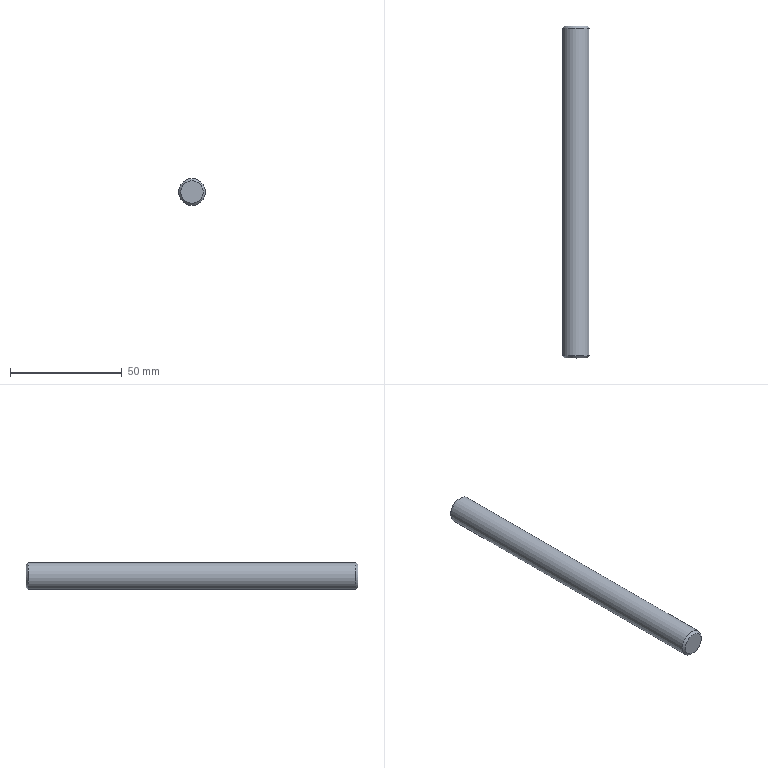Part | NX | features solid 2 | 1 solid | 5 faces | box 12 x 148.5 x 12 mm | volume 16759 mm3 | plane 2 | cone 2 | cylinder 1 | commonest cylinder face diameters 12 x1
STEP:
#1=CARTESIAN_POINT('',(0.,611.5,-123.));
#2=VERTEX_POINT('',#1);
#3=CARTESIAN_POINT('',(0.,611.5,-117.));
#4=DIRECTION('',(0.,-1.,0.));
#5=DIRECTION('',(0.,0.,-1.));
#6=AXIS2_PLACEMENT_3D('',#3,#4,#5);
#7=CIRCLE('',#6,6.);
#8=EDGE_CURVE('',#2,#2,#7,.F.);
#9=ORIENTED_EDGE('',*,*,#8,.T.);
#10=EDGE_LOOP('',(#9));
#11=FACE_BOUND('',#10,.T.);
#12=CARTESIAN_POINT('',(0.,758.,-123.));
#13=VERTEX_POINT('',#12);
#14=CARTESIAN_POINT('',(0.,758.,-117.));
#15=DIRECTION('',(0.,-1.,0.));
#16=DIRECTION('',(0.,0.,-1.));
#17=AXIS2_PLACEMENT_3D('',#14,#15,#16);
#18=CIRCLE('',#17,6.);
#19=EDGE_CURVE('',#13,#13,#18,.T.);
#20=ORIENTED_EDGE('',*,*,#19,.T.);
#21=EDGE_LOOP('',(#20));
#22=FACE_BOUND('',#21,.T.);
#23=CARTESIAN_POINT('',(0.,611.,-117.));
#24=DIRECTION('',(0.,1.,0.));
#25=DIRECTION('',(0.,0.,1.));
#26=AXIS2_PLACEMENT_3D('',#23,#24,#25);
#27=CYLINDRICAL_SURFACE('',#26,6.);
#28=ADVANCED_FACE('',(#11,#22),#27,.T.);
#29=CARTESIAN_POINT('',(0.,610.5,-122.));
#30=VERTEX_POINT('',#29);
#31=CARTESIAN_POINT('',(0.,610.5,-117.));
#32=DIRECTION('',(0.,-1.,0.));
#33=DIRECTION('',(0.,0.,-1.));
#34=AXIS2_PLACEMENT_3D('',#31,#32,#33);
#35=CIRCLE('',#34,5.);
#36=EDGE_CURVE('',#30,#30,#35,.T.);
#37=ORIENTED_EDGE('',*,*,#36,.T.);
#38=EDGE_LOOP('',(#37));
#39=FACE_BOUND('',#38,.T.);
#40=CARTESIAN_POINT('',(0.,610.5,-117.));
#41=DIRECTION('',(0.,-1.,0.));
#42=DIRECTION('',(0.,0.,-1.));
#43=AXIS2_PLACEMENT_3D('',#40,#41,#42);
#44=PLANE('',#43);
#45=ADVANCED_FACE('',(#39),#44,.T.);
#46=CARTESIAN_POINT('',(0.,759.,-122.));
#47=VERTEX_POINT('',#46);
#48=CARTESIAN_POINT('',(0.,759.,-117.));
#49=DIRECTION('',(0.,-1.,0.));
#50=DIRECTION('',(0.,0.,-1.));
#51=AXIS2_PLACEMENT_3D('',#48,#49,#50);
#52=CIRCLE('',#51,5.);
#53=EDGE_CURVE('',#47,#47,#52,.F.);
#54=ORIENTED_EDGE('',*,*,#53,.T.);
#55=EDGE_LOOP('',(#54));
#56=FACE_BOUND('',#55,.T.);
#57=CARTESIAN_POINT('',(0.,759.,-117.));
#58=DIRECTION('',(0.,-1.,0.));
#59=DIRECTION('',(0.,0.,-1.));
#60=AXIS2_PLACEMENT_3D('',#57,#58,#59);
#61=PLANE('',#60);
#62=ADVANCED_FACE('',(#56),#61,.F.);
#63=ORIENTED_EDGE('',*,*,#8,.F.);
#64=EDGE_LOOP('',(#63));
#65=FACE_BOUND('',#64,.T.);
#66=ORIENTED_EDGE('',*,*,#36,.F.);
#67=EDGE_LOOP('',(#66));
#68=FACE_BOUND('',#67,.T.);
#69=CARTESIAN_POINT('',(0.,610.5,-117.));
#70=DIRECTION('',(0.,1.,0.));
#71=DIRECTION('',(0.,0.,1.));
#72=AXIS2_PLACEMENT_3D('',#69,#70,#71);
#73=CONICAL_SURFACE('',#72,5.,0.7854);
#74=ADVANCED_FACE('',(#65,#68),#73,.T.);
#75=ORIENTED_EDGE('',*,*,#53,.F.);
#76=EDGE_LOOP('',(#75));
#77=FACE_BOUND('',#76,.T.);
#78=ORIENTED_EDGE('',*,*,#19,.F.);
#79=EDGE_LOOP('',(#78));
#80=FACE_BOUND('',#79,.T.);
#81=CARTESIAN_POINT('',(0.,758.,-117.));
#82=DIRECTION('',(0.,-1.,0.));
#83=DIRECTION('',(0.,0.,-1.));
#84=AXIS2_PLACEMENT_3D('',#81,#82,#83);
#85=CONICAL_SURFACE('',#84,6.,0.7854);
#86=ADVANCED_FACE('',(#77,#80),#85,.T.);
#87=CLOSED_SHELL('',(#28,#45,#62,#74,#86));
#88=MANIFOLD_SOLID_BREP('',#87);
#89=(LENGTH_UNIT()NAMED_UNIT(*)SI_UNIT(.MILLI.,.METRE.));
#90=UNCERTAINTY_MEASURE_WITH_UNIT(LENGTH_MEASURE(0.00001),#89,'','');
#91=(NAMED_UNIT(*)PLANE_ANGLE_UNIT()SI_UNIT($,.RADIAN.));
#92=(NAMED_UNIT(*)SI_UNIT($,.STERADIAN.)SOLID_ANGLE_UNIT());
#93=(GEOMETRIC_REPRESENTATION_CONTEXT(3)GLOBAL_UNCERTAINTY_ASSIGNED_CONTEXT((#90))GLOBAL_UNIT_ASSIGNED_CONTEXT((#89,#91,#92))REPRESENTATION_CONTEXT('',''));
#94=ADVANCED_BREP_SHAPE_REPRESENTATION('',(#88),#93);